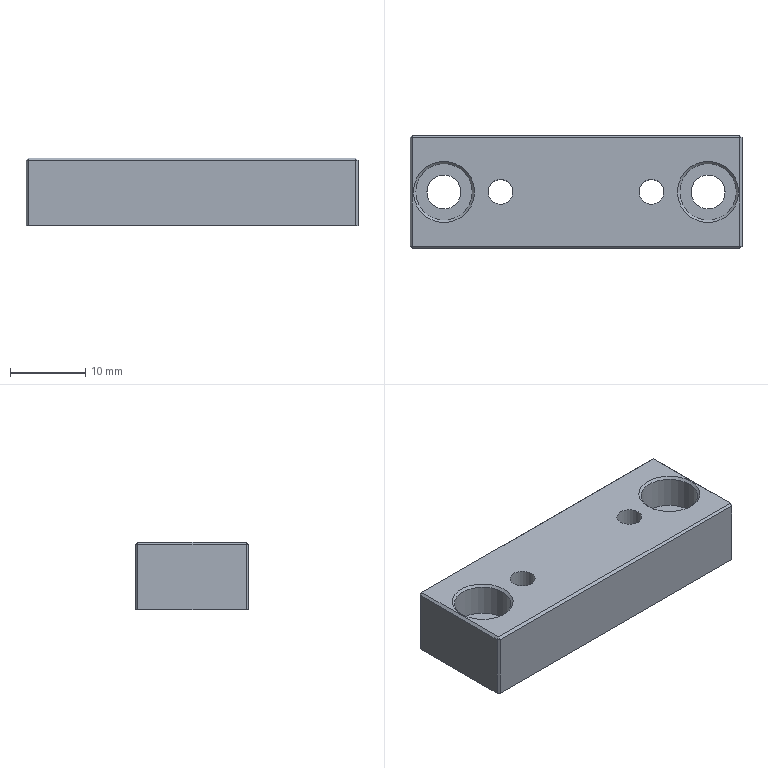CAM job | NX | 3-axis milling, drilling | part box 44 x 15 x 9 mm | stock box 49 x 20 x 12 mm
Tools:
number,name,description,diameter,corner_radius,flute_length,length,flutes
4,D4,平底铣刀-粗,4.0,0.0,25.0,75.0,2
9,D10,平底铣刀-粗,10.0,0.0,35.0,75.0,2
10,D10-J,平底铣刀-精,10.0,0.0,35.0,75.0,2
1,D80R0.8飞刀,圆鼻刀-粗,80.0,0.8,50.0,75.0,2
2,D6倒角刀,倒角刀,6.0,0.0,3.0,25.0,2
21,M4X0.7,丝锥,3.3,0.0,35.0,50.0,2
11,ZT4.5,钻头,4.5,0.0,35.0,50.0,2
13,钻头3.3,Twist Drill 3.3 mm,3.3,0.0,35.0,35.008,2
Operations:
program,operation,operation_type,tool,method,geometry_group,spindle_rpm,surface_speed,feed_per_tooth,feed_cut,feed_plunge,cut_length_mm,path_length_mm,cut_time_min,machine_time_min
A,顶面,FaceMilling,D80R0.8飞刀,侧刃精光-切深K-步距G,W-A,4000.0,1005.31,0.125,1000.0,100.0,138.0,174.0,0.138,0.1416
A,外形粗_2,VolumeBased25DMillingOperation,D10,METHOD,W-A,8000.0,251.327,0.3125,5000.0,80.0,2092.302,2140.002,0.4185,0.4232
A,打点-深0.8,Operation,D6倒角刀,NONE,W-A,8000.0,150.796,0.0312,500.0,90.0,7.2,92.558,0.0144,0.0229
A,通孔-M4螺纹底孔,Operation,钻头3.3,NONE,W-A,3000.0,31.102,0.05,300.0,90.0,31.983,124.991,0.1066,0.1159
A,沉头孔-钻孔0段,Operation,ZT4.5,NONE,W-A,2800.0,39.584,0.0179,100.0,90.0,26.704,129.422,0.267,0.2773
A,铣孔开粗D4_1,CylinderMilling,D4,NONE,W-A,8000.0,100.531,0.075,1200.0,100.0,397.565,519.965,0.3313,0.3435
A,铣孔精光D4_1,CylinderMilling,D4,精光步距切深关,W-A,8000.0,100.531,0.0312,500.0,100.0,58.465,180.864,0.1169,0.1292
A,钻倒角_1,Operation,D6倒角刀,METHOD,W-A,8000.0,150.796,0.0312,500.0,0.0,10.4,84.024,0.0208,0.0282
A,铣倒角_1,PlanarMilling,D6倒角刀,NONE,W-A,8000.0,150.796,0.0312,500.0,100.0,62.778,175.284,0.1256,0.1368
A,底壁铣倒角_COPY,VolumeBased25DMillingOperation,D6倒角刀,爬面_倒角-切深0-步距G,W-A,6500.0,122.519,0.1154,1500.0,100.0,130.77,169.77,0.0872,0.0911
A,通孔-攻牙M4,Operation,M4X0.7,METHOD,W-A,600.0,6.22,0.0006,0.7,90.0,26.0,113.025,37.143,37.152
A,外形半精_2,VolumeBased25DMillingOperation,D10-J,METHOD,W-A,8000.0,251.327,0.0625,1000.0,100.0,153.671,211.071,0.1537,0.1594